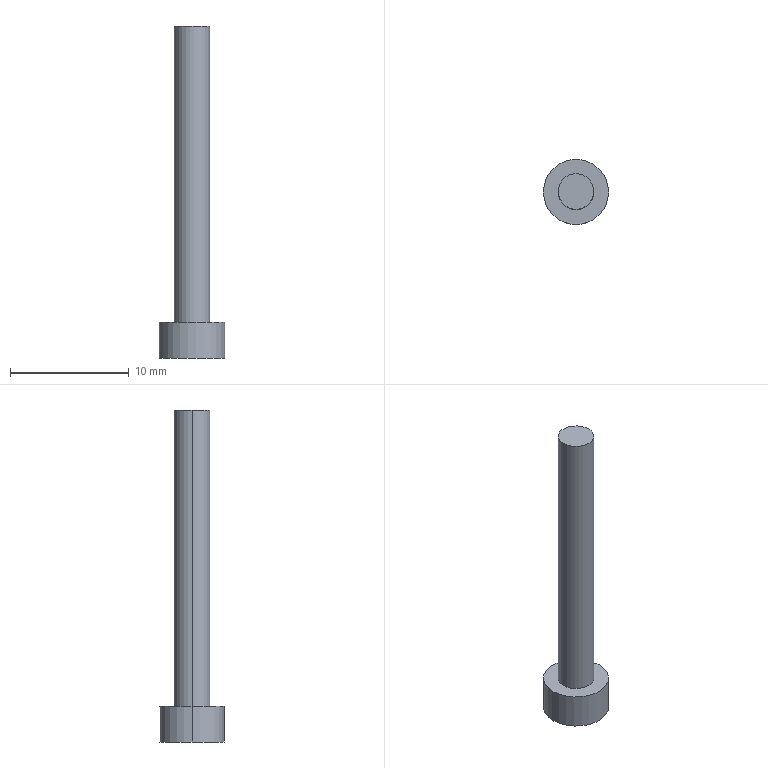Part | STEP file | M3 long screw | 1 solid | 7 faces | box 5.5 x 5.5 x 28 mm | volume 247.989 mm3 | cylinder 4 | plane 3 | commonest cylinder face diameters 3 x2 5.5 x2
STEP:
#1=CARTESIAN_POINT('',(0.,0.,0.));
#2=DIRECTION('',(0.,0.,1.));
#3=DIRECTION('',(1.,0.,0.));
#4=AXIS2_PLACEMENT_3D('',#1,#2,#3);
#5=CARTESIAN_POINT('',(1.5,0.,28.));
#6=VERTEX_POINT('',#5);
#7=CARTESIAN_POINT('',(-1.5,0.,28.));
#8=VERTEX_POINT('',#7);
#9=CARTESIAN_POINT('',(0.,0.,28.));
#10=DIRECTION('',(0.,0.,1.));
#11=DIRECTION('',(1.,0.,0.));
#12=AXIS2_PLACEMENT_3D('',#9,#10,#11);
#13=CIRCLE('',#12,1.5);
#14=CARTESIAN_POINT('',(0.,0.,28.));
#15=DIRECTION('',(0.,0.,-1.));
#16=DIRECTION('',(-1.,0.,0.));
#17=AXIS2_PLACEMENT_3D('',#14,#15,#16);
#18=CYLINDRICAL_SURFACE('',#17,1.5);
#19=CARTESIAN_POINT('',(3.142,0.));
#20=DIRECTION('',(-1.,0.));
#21=VECTOR('',#20,1.);
#22=LINE('',#19,#21);
#23=(GEOMETRIC_REPRESENTATION_CONTEXT(2)PARAMETRIC_REPRESENTATION_CONTEXT()REPRESENTATION_CONTEXT('',''));
#24=DEFINITIONAL_REPRESENTATION('',(#22),#23);
#25=PCURVE('',#18,#24);
#26=CARTESIAN_POINT('',(0.,0.,28.));
#27=DIRECTION('',(0.,0.,1.));
#28=DIRECTION('',(1.,0.,0.));
#29=AXIS2_PLACEMENT_3D('',#26,#27,#28);
#30=PLANE('',#29);
#31=CARTESIAN_POINT('',(0.,0.));
#32=DIRECTION('',(1.,0.));
#33=AXIS2_PLACEMENT_2D('',#31,#32);
#34=CIRCLE('',#33,1.5);
#35=(GEOMETRIC_REPRESENTATION_CONTEXT(2)PARAMETRIC_REPRESENTATION_CONTEXT()REPRESENTATION_CONTEXT('',''));
#36=DEFINITIONAL_REPRESENTATION('',(#34),#35);
#37=PCURVE('',#30,#36);
#38=SURFACE_CURVE('',#13,(#25,#37),.PCURVE_S1.);
#39=EDGE_CURVE('',#6,#8,#38,.T.);
#40=ORIENTED_EDGE('',*,*,#39,.F.);
#41=CARTESIAN_POINT('',(1.5,0.,3.));
#42=VERTEX_POINT('',#41);
#43=CARTESIAN_POINT('',(1.5,0.,28.));
#44=DIRECTION('',(0.,0.,-1.));
#45=VECTOR('',#44,1.);
#46=LINE('',#43,#45);
#47=CARTESIAN_POINT('',(3.142,0.));
#48=DIRECTION('',(0.,1.));
#49=VECTOR('',#48,1.);
#50=LINE('',#47,#49);
#51=(GEOMETRIC_REPRESENTATION_CONTEXT(2)PARAMETRIC_REPRESENTATION_CONTEXT()REPRESENTATION_CONTEXT('',''));
#52=DEFINITIONAL_REPRESENTATION('',(#50),#51);
#53=PCURVE('',#18,#52);
#54=CARTESIAN_POINT('',(0.,0.,28.));
#55=DIRECTION('',(0.,0.,-1.));
#56=DIRECTION('',(-1.,0.,0.));
#57=AXIS2_PLACEMENT_3D('',#54,#55,#56);
#58=CYLINDRICAL_SURFACE('',#57,1.5);
#59=CARTESIAN_POINT('',(3.142,0.));
#60=DIRECTION('',(0.,1.));
#61=VECTOR('',#60,1.);
#62=LINE('',#59,#61);
#63=(GEOMETRIC_REPRESENTATION_CONTEXT(2)PARAMETRIC_REPRESENTATION_CONTEXT()REPRESENTATION_CONTEXT('',''));
#64=DEFINITIONAL_REPRESENTATION('',(#62),#63);
#65=PCURVE('',#58,#64);
#66=SURFACE_CURVE('',#46,(#53,#65),.PCURVE_S1.);
#67=EDGE_CURVE('',#6,#42,#66,.T.);
#68=ORIENTED_EDGE('',*,*,#67,.T.);
#69=CARTESIAN_POINT('',(-1.5,0.,3.));
#70=VERTEX_POINT('',#69);
#71=CARTESIAN_POINT('',(0.,0.,3.));
#72=DIRECTION('',(0.,0.,1.));
#73=DIRECTION('',(1.,0.,0.));
#74=AXIS2_PLACEMENT_3D('',#71,#72,#73);
#75=CIRCLE('',#74,1.5);
#76=CARTESIAN_POINT('',(3.142,25.));
#77=DIRECTION('',(-1.,0.));
#78=VECTOR('',#77,1.);
#79=LINE('',#76,#78);
#80=(GEOMETRIC_REPRESENTATION_CONTEXT(2)PARAMETRIC_REPRESENTATION_CONTEXT()REPRESENTATION_CONTEXT('',''));
#81=DEFINITIONAL_REPRESENTATION('',(#79),#80);
#82=PCURVE('',#18,#81);
#83=CARTESIAN_POINT('',(0.,0.,3.));
#84=DIRECTION('',(0.,0.,1.));
#85=DIRECTION('',(1.,0.,0.));
#86=AXIS2_PLACEMENT_3D('',#83,#84,#85);
#87=PLANE('',#86);
#88=CARTESIAN_POINT('',(0.,0.));
#89=DIRECTION('',(1.,0.));
#90=AXIS2_PLACEMENT_2D('',#88,#89);
#91=CIRCLE('',#90,1.5);
#92=(GEOMETRIC_REPRESENTATION_CONTEXT(2)PARAMETRIC_REPRESENTATION_CONTEXT()REPRESENTATION_CONTEXT('',''));
#93=DEFINITIONAL_REPRESENTATION('',(#91),#92);
#94=PCURVE('',#87,#93);
#95=SURFACE_CURVE('',#75,(#82,#94),.PCURVE_S1.);
#96=EDGE_CURVE('',#42,#70,#95,.T.);
#97=ORIENTED_EDGE('',*,*,#96,.T.);
#98=CARTESIAN_POINT('',(-1.5,0.,28.));
#99=DIRECTION('',(0.,0.,-1.));
#100=VECTOR('',#99,1.);
#101=LINE('',#98,#100);
#102=CARTESIAN_POINT('',(0.,0.));
#103=DIRECTION('',(0.,1.));
#104=VECTOR('',#103,1.);
#105=LINE('',#102,#104);
#106=(GEOMETRIC_REPRESENTATION_CONTEXT(2)PARAMETRIC_REPRESENTATION_CONTEXT()REPRESENTATION_CONTEXT('',''));
#107=DEFINITIONAL_REPRESENTATION('',(#105),#106);
#108=PCURVE('',#18,#107);
#109=CARTESIAN_POINT('',(6.283,0.));
#110=DIRECTION('',(0.,1.));
#111=VECTOR('',#110,1.);
#112=LINE('',#109,#111);
#113=(GEOMETRIC_REPRESENTATION_CONTEXT(2)PARAMETRIC_REPRESENTATION_CONTEXT()REPRESENTATION_CONTEXT('',''));
#114=DEFINITIONAL_REPRESENTATION('',(#112),#113);
#115=PCURVE('',#58,#114);
#116=SURFACE_CURVE('',#101,(#108,#115),.PCURVE_S1.);
#117=EDGE_CURVE('',#8,#70,#116,.T.);
#118=ORIENTED_EDGE('',*,*,#117,.F.);
#119=EDGE_LOOP('',(#40,#68,#97,#118));
#120=FACE_BOUND('',#119,.T.);
#121=ADVANCED_FACE('',(#120),#18,.T.);
#122=CARTESIAN_POINT('',(2.75,0.,3.));
#123=VERTEX_POINT('',#122);
#124=CARTESIAN_POINT('',(-2.75,0.,3.));
#125=VERTEX_POINT('',#124);
#126=CARTESIAN_POINT('',(0.,0.,3.));
#127=DIRECTION('',(0.,0.,1.));
#128=DIRECTION('',(1.,0.,0.));
#129=AXIS2_PLACEMENT_3D('',#126,#127,#128);
#130=CIRCLE('',#129,2.75);
#131=CARTESIAN_POINT('',(0.,0.,3.));
#132=DIRECTION('',(0.,0.,-1.));
#133=DIRECTION('',(-1.,0.,0.));
#134=AXIS2_PLACEMENT_3D('',#131,#132,#133);
#135=CYLINDRICAL_SURFACE('',#134,2.75);
#136=CARTESIAN_POINT('',(3.142,0.));
#137=DIRECTION('',(-1.,0.));
#138=VECTOR('',#137,1.);
#139=LINE('',#136,#138);
#140=(GEOMETRIC_REPRESENTATION_CONTEXT(2)PARAMETRIC_REPRESENTATION_CONTEXT()REPRESENTATION_CONTEXT('',''));
#141=DEFINITIONAL_REPRESENTATION('',(#139),#140);
#142=PCURVE('',#135,#141);
#143=CARTESIAN_POINT('',(0.,0.));
#144=DIRECTION('',(1.,0.));
#145=AXIS2_PLACEMENT_2D('',#143,#144);
#146=CIRCLE('',#145,2.75);
#147=(GEOMETRIC_REPRESENTATION_CONTEXT(2)PARAMETRIC_REPRESENTATION_CONTEXT()REPRESENTATION_CONTEXT('',''));
#148=DEFINITIONAL_REPRESENTATION('',(#146),#147);
#149=PCURVE('',#87,#148);
#150=SURFACE_CURVE('',#130,(#142,#149),.PCURVE_S1.);
#151=EDGE_CURVE('',#123,#125,#150,.T.);
#152=ORIENTED_EDGE('',*,*,#151,.F.);
#153=CARTESIAN_POINT('',(2.75,0.,0.));
#154=VERTEX_POINT('',#153);
#155=CARTESIAN_POINT('',(2.75,0.,3.));
#156=DIRECTION('',(0.,0.,-1.));
#157=VECTOR('',#156,1.);
#158=LINE('',#155,#157);
#159=CARTESIAN_POINT('',(3.142,0.));
#160=DIRECTION('',(0.,1.));
#161=VECTOR('',#160,1.);
#162=LINE('',#159,#161);
#163=(GEOMETRIC_REPRESENTATION_CONTEXT(2)PARAMETRIC_REPRESENTATION_CONTEXT()REPRESENTATION_CONTEXT('',''));
#164=DEFINITIONAL_REPRESENTATION('',(#162),#163);
#165=PCURVE('',#135,#164);
#166=CARTESIAN_POINT('',(0.,0.,3.));
#167=DIRECTION('',(0.,0.,-1.));
#168=DIRECTION('',(-1.,0.,0.));
#169=AXIS2_PLACEMENT_3D('',#166,#167,#168);
#170=CYLINDRICAL_SURFACE('',#169,2.75);
#171=CARTESIAN_POINT('',(3.142,0.));
#172=DIRECTION('',(0.,1.));
#173=VECTOR('',#172,1.);
#174=LINE('',#171,#173);
#175=(GEOMETRIC_REPRESENTATION_CONTEXT(2)PARAMETRIC_REPRESENTATION_CONTEXT()REPRESENTATION_CONTEXT('',''));
#176=DEFINITIONAL_REPRESENTATION('',(#174),#175);
#177=PCURVE('',#170,#176);
#178=SURFACE_CURVE('',#158,(#165,#177),.PCURVE_S1.);
#179=EDGE_CURVE('',#123,#154,#178,.T.);
#180=ORIENTED_EDGE('',*,*,#179,.T.);
#181=CARTESIAN_POINT('',(-2.75,0.,0.));
#182=VERTEX_POINT('',#181);
#183=CARTESIAN_POINT('',(0.,0.,0.));
#184=DIRECTION('',(0.,0.,1.));
#185=DIRECTION('',(1.,0.,0.));
#186=AXIS2_PLACEMENT_3D('',#183,#184,#185);
#187=CIRCLE('',#186,2.75);
#188=CARTESIAN_POINT('',(3.142,3.));
#189=DIRECTION('',(-1.,0.));
#190=VECTOR('',#189,1.);
#191=LINE('',#188,#190);
#192=(GEOMETRIC_REPRESENTATION_CONTEXT(2)PARAMETRIC_REPRESENTATION_CONTEXT()REPRESENTATION_CONTEXT('',''));
#193=DEFINITIONAL_REPRESENTATION('',(#191),#192);
#194=PCURVE('',#135,#193);
#195=CARTESIAN_POINT('',(0.,0.,0.));
#196=DIRECTION('',(0.,0.,1.));
#197=DIRECTION('',(1.,0.,0.));
#198=AXIS2_PLACEMENT_3D('',#195,#196,#197);
#199=PLANE('',#198);
#200=CARTESIAN_POINT('',(0.,0.));
#201=DIRECTION('',(1.,0.));
#202=AXIS2_PLACEMENT_2D('',#200,#201);
#203=CIRCLE('',#202,2.75);
#204=(GEOMETRIC_REPRESENTATION_CONTEXT(2)PARAMETRIC_REPRESENTATION_CONTEXT()REPRESENTATION_CONTEXT('',''));
#205=DEFINITIONAL_REPRESENTATION('',(#203),#204);
#206=PCURVE('',#199,#205);
#207=SURFACE_CURVE('',#187,(#194,#206),.PCURVE_S1.);
#208=EDGE_CURVE('',#154,#182,#207,.T.);
#209=ORIENTED_EDGE('',*,*,#208,.T.);
#210=CARTESIAN_POINT('',(-2.75,0.,3.));
#211=DIRECTION('',(0.,0.,-1.));
#212=VECTOR('',#211,1.);
#213=LINE('',#210,#212);
#214=CARTESIAN_POINT('',(0.,0.));
#215=DIRECTION('',(0.,1.));
#216=VECTOR('',#215,1.);
#217=LINE('',#214,#216);
#218=(GEOMETRIC_REPRESENTATION_CONTEXT(2)PARAMETRIC_REPRESENTATION_CONTEXT()REPRESENTATION_CONTEXT('',''));
#219=DEFINITIONAL_REPRESENTATION('',(#217),#218);
#220=PCURVE('',#135,#219);
#221=CARTESIAN_POINT('',(6.283,0.));
#222=DIRECTION('',(0.,1.));
#223=VECTOR('',#222,1.);
#224=LINE('',#221,#223);
#225=(GEOMETRIC_REPRESENTATION_CONTEXT(2)PARAMETRIC_REPRESENTATION_CONTEXT()REPRESENTATION_CONTEXT('',''));
#226=DEFINITIONAL_REPRESENTATION('',(#224),#225);
#227=PCURVE('',#170,#226);
#228=SURFACE_CURVE('',#213,(#220,#227),.PCURVE_S1.);
#229=EDGE_CURVE('',#125,#182,#228,.T.);
#230=ORIENTED_EDGE('',*,*,#229,.F.);
#231=EDGE_LOOP('',(#152,#180,#209,#230));
#232=FACE_BOUND('',#231,.T.);
#233=ADVANCED_FACE('',(#232),#135,.T.);
#234=CARTESIAN_POINT('',(0.,0.,3.));
#235=DIRECTION('',(0.,0.,1.));
#236=DIRECTION('',(1.,0.,0.));
#237=AXIS2_PLACEMENT_3D('',#234,#235,#236);
#238=CIRCLE('',#237,2.75);
#239=CARTESIAN_POINT('',(0.,0.));
#240=DIRECTION('',(1.,0.));
#241=AXIS2_PLACEMENT_2D('',#239,#240);
#242=CIRCLE('',#241,2.75);
#243=(GEOMETRIC_REPRESENTATION_CONTEXT(2)PARAMETRIC_REPRESENTATION_CONTEXT()REPRESENTATION_CONTEXT('',''));
#244=DEFINITIONAL_REPRESENTATION('',(#242),#243);
#245=PCURVE('',#87,#244);
#246=CARTESIAN_POINT('',(9.425,0.));
#247=DIRECTION('',(-1.,0.));
#248=VECTOR('',#247,1.);
#249=LINE('',#246,#248);
#250=(GEOMETRIC_REPRESENTATION_CONTEXT(2)PARAMETRIC_REPRESENTATION_CONTEXT()REPRESENTATION_CONTEXT('',''));
#251=DEFINITIONAL_REPRESENTATION('',(#249),#250);
#252=PCURVE('',#170,#251);
#253=SURFACE_CURVE('',#238,(#245,#252),.PCURVE_S1.);
#254=EDGE_CURVE('',#125,#123,#253,.T.);
#255=ORIENTED_EDGE('',*,*,#254,.T.);
#256=ORIENTED_EDGE('',*,*,#151,.T.);
#257=EDGE_LOOP('',(#255,#256));
#258=FACE_BOUND('',#257,.T.);
#259=CARTESIAN_POINT('',(0.,0.,3.));
#260=DIRECTION('',(0.,0.,1.));
#261=DIRECTION('',(1.,0.,0.));
#262=AXIS2_PLACEMENT_3D('',#259,#260,#261);
#263=CIRCLE('',#262,1.5);
#264=CARTESIAN_POINT('',(0.,0.));
#265=DIRECTION('',(1.,0.));
#266=AXIS2_PLACEMENT_2D('',#264,#265);
#267=CIRCLE('',#266,1.5);
#268=(GEOMETRIC_REPRESENTATION_CONTEXT(2)PARAMETRIC_REPRESENTATION_CONTEXT()REPRESENTATION_CONTEXT('',''));
#269=DEFINITIONAL_REPRESENTATION('',(#267),#268);
#270=PCURVE('',#87,#269);
#271=CARTESIAN_POINT('',(9.425,25.));
#272=DIRECTION('',(-1.,0.));
#273=VECTOR('',#272,1.);
#274=LINE('',#271,#273);
#275=(GEOMETRIC_REPRESENTATION_CONTEXT(2)PARAMETRIC_REPRESENTATION_CONTEXT()REPRESENTATION_CONTEXT('',''));
#276=DEFINITIONAL_REPRESENTATION('',(#274),#275);
#277=PCURVE('',#58,#276);
#278=SURFACE_CURVE('',#263,(#270,#277),.PCURVE_S1.);
#279=EDGE_CURVE('',#70,#42,#278,.T.);
#280=ORIENTED_EDGE('',*,*,#279,.F.);
#281=ORIENTED_EDGE('',*,*,#96,.F.);
#282=EDGE_LOOP('',(#280,#281));
#283=FACE_BOUND('',#282,.T.);
#284=ADVANCED_FACE('',(#258,#283),#87,.T.);
#285=ORIENTED_EDGE('',*,*,#179,.F.);
#286=ORIENTED_EDGE('',*,*,#254,.F.);
#287=ORIENTED_EDGE('',*,*,#229,.T.);
#288=CARTESIAN_POINT('',(0.,0.,0.));
#289=DIRECTION('',(0.,0.,1.));
#290=DIRECTION('',(1.,0.,0.));
#291=AXIS2_PLACEMENT_3D('',#288,#289,#290);
#292=CIRCLE('',#291,2.75);
#293=CARTESIAN_POINT('',(9.425,3.));
#294=DIRECTION('',(-1.,0.));
#295=VECTOR('',#294,1.);
#296=LINE('',#293,#295);
#297=(GEOMETRIC_REPRESENTATION_CONTEXT(2)PARAMETRIC_REPRESENTATION_CONTEXT()REPRESENTATION_CONTEXT('',''));
#298=DEFINITIONAL_REPRESENTATION('',(#296),#297);
#299=PCURVE('',#170,#298);
#300=CARTESIAN_POINT('',(0.,0.));
#301=DIRECTION('',(1.,0.));
#302=AXIS2_PLACEMENT_2D('',#300,#301);
#303=CIRCLE('',#302,2.75);
#304=(GEOMETRIC_REPRESENTATION_CONTEXT(2)PARAMETRIC_REPRESENTATION_CONTEXT()REPRESENTATION_CONTEXT('',''));
#305=DEFINITIONAL_REPRESENTATION('',(#303),#304);
#306=PCURVE('',#199,#305);
#307=SURFACE_CURVE('',#292,(#299,#306),.PCURVE_S1.);
#308=EDGE_CURVE('',#182,#154,#307,.T.);
#309=ORIENTED_EDGE('',*,*,#308,.T.);
#310=EDGE_LOOP('',(#285,#286,#287,#309));
#311=FACE_BOUND('',#310,.T.);
#312=ADVANCED_FACE('',(#311),#170,.T.);
#313=ORIENTED_EDGE('',*,*,#308,.F.);
#314=ORIENTED_EDGE('',*,*,#208,.F.);
#315=EDGE_LOOP('',(#313,#314));
#316=FACE_BOUND('',#315,.T.);
#317=ADVANCED_FACE('',(#316),#199,.F.);
#318=ORIENTED_EDGE('',*,*,#67,.F.);
#319=CARTESIAN_POINT('',(0.,0.,28.));
#320=DIRECTION('',(0.,0.,1.));
#321=DIRECTION('',(1.,0.,0.));
#322=AXIS2_PLACEMENT_3D('',#319,#320,#321);
#323=CIRCLE('',#322,1.5);
#324=CARTESIAN_POINT('',(9.425,0.));
#325=DIRECTION('',(-1.,0.));
#326=VECTOR('',#325,1.);
#327=LINE('',#324,#326);
#328=(GEOMETRIC_REPRESENTATION_CONTEXT(2)PARAMETRIC_REPRESENTATION_CONTEXT()REPRESENTATION_CONTEXT('',''));
#329=DEFINITIONAL_REPRESENTATION('',(#327),#328);
#330=PCURVE('',#58,#329);
#331=CARTESIAN_POINT('',(0.,0.));
#332=DIRECTION('',(1.,0.));
#333=AXIS2_PLACEMENT_2D('',#331,#332);
#334=CIRCLE('',#333,1.5);
#335=(GEOMETRIC_REPRESENTATION_CONTEXT(2)PARAMETRIC_REPRESENTATION_CONTEXT()REPRESENTATION_CONTEXT('',''));
#336=DEFINITIONAL_REPRESENTATION('',(#334),#335);
#337=PCURVE('',#30,#336);
#338=SURFACE_CURVE('',#323,(#330,#337),.PCURVE_S1.);
#339=EDGE_CURVE('',#8,#6,#338,.T.);
#340=ORIENTED_EDGE('',*,*,#339,.F.);
#341=ORIENTED_EDGE('',*,*,#117,.T.);
#342=ORIENTED_EDGE('',*,*,#279,.T.);
#343=EDGE_LOOP('',(#318,#340,#341,#342));
#344=FACE_BOUND('',#343,.T.);
#345=ADVANCED_FACE('',(#344),#58,.T.);
#346=ORIENTED_EDGE('',*,*,#339,.T.);
#347=ORIENTED_EDGE('',*,*,#39,.T.);
#348=EDGE_LOOP('',(#346,#347));
#349=FACE_BOUND('',#348,.T.);
#350=ADVANCED_FACE('',(#349),#30,.T.);
#351=CLOSED_SHELL('',(#121,#233,#284,#312,#317,#345,#350));
#352=MANIFOLD_SOLID_BREP('',#351);
#353=(LENGTH_UNIT()NAMED_UNIT(*)SI_UNIT(.MILLI.,.METRE.));
#354=UNCERTAINTY_MEASURE_WITH_UNIT(LENGTH_MEASURE(0.0000001),#353,'','');
#355=(NAMED_UNIT(*)PLANE_ANGLE_UNIT()SI_UNIT($,.RADIAN.));
#356=(NAMED_UNIT(*)SI_UNIT($,.STERADIAN.)SOLID_ANGLE_UNIT());
#357=(GEOMETRIC_REPRESENTATION_CONTEXT(3)GLOBAL_UNCERTAINTY_ASSIGNED_CONTEXT((#354))GLOBAL_UNIT_ASSIGNED_CONTEXT((#353,#355,#356))REPRESENTATION_CONTEXT('',''));
#358=ADVANCED_BREP_SHAPE_REPRESENTATION('',(#4,#352),#357);